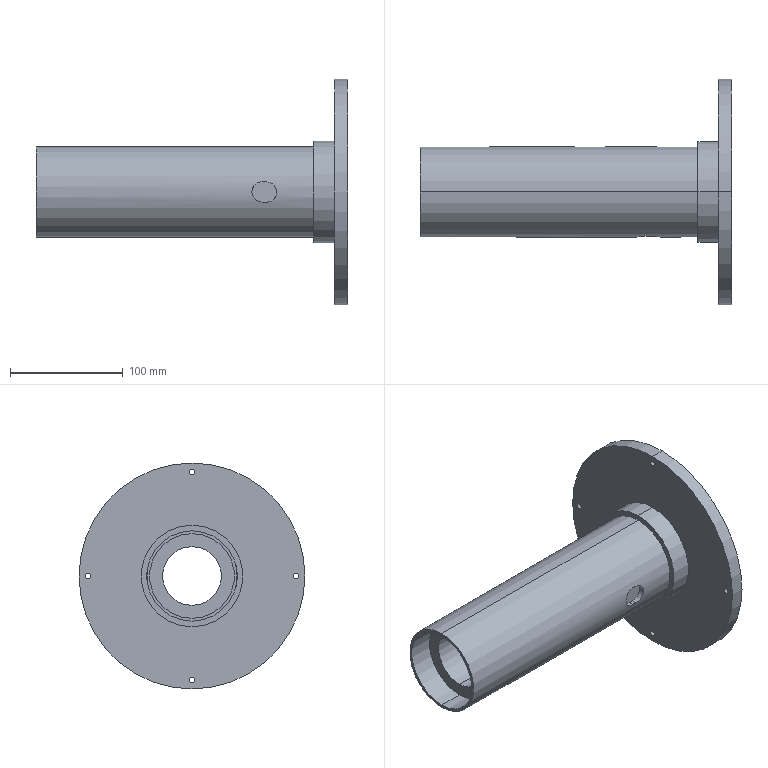Part | NX | features BREP 1 | 1 solid | 36 faces | box 276 x 200 x 200 mm | volume 1052758 mm3 | cylinder 24 | plane 12 | commonest cylinder face diameters 5 x8 9 x2 18 x2 52 x2 72 x2 75 x2
STEP:
#1=CARTESIAN_POINT('',(169.294,92.,2.5));
#2=VERTEX_POINT('',#1);
#3=CARTESIAN_POINT('',(169.294,92.,-2.5));
#4=VERTEX_POINT('',#3);
#5=CARTESIAN_POINT('',(169.294,92.,0.));
#6=DIRECTION('',(1.,0.,0.));
#7=DIRECTION('',(0.,0.,-1.));
#8=AXIS2_PLACEMENT_3D('',#5,#6,#7);
#9=CIRCLE('',#8,2.5);
#10=EDGE_CURVE('',#2,#4,#9,.T.);
#11=ORIENTED_EDGE('',*,*,#10,.F.);
#12=CARTESIAN_POINT('',(181.294,92.,2.5));
#13=VERTEX_POINT('',#12);
#14=CARTESIAN_POINT('',(181.294,92.,2.5));
#15=DIRECTION('',(1.,0.,0.));
#16=VECTOR('',#15,1000.);
#17=LINE('',#14,#16);
#18=EDGE_CURVE('',#13,#2,#17,.F.);
#19=ORIENTED_EDGE('',*,*,#18,.F.);
#20=CARTESIAN_POINT('',(181.294,92.,-2.5));
#21=VERTEX_POINT('',#20);
#22=CARTESIAN_POINT('',(181.294,92.,0.));
#23=DIRECTION('',(1.,0.,0.));
#24=DIRECTION('',(0.,0.,-1.));
#25=AXIS2_PLACEMENT_3D('',#22,#23,#24);
#26=CIRCLE('',#25,2.5);
#27=EDGE_CURVE('',#13,#21,#26,.T.);
#28=ORIENTED_EDGE('',*,*,#27,.T.);
#29=CARTESIAN_POINT('',(181.294,92.,-2.5));
#30=DIRECTION('',(1.,0.,0.));
#31=VECTOR('',#30,1000.);
#32=LINE('',#29,#31);
#33=EDGE_CURVE('',#21,#4,#32,.F.);
#34=ORIENTED_EDGE('',*,*,#33,.T.);
#35=EDGE_LOOP('',(#11,#19,#28,#34));
#36=FACE_BOUND('',#35,.T.);
#37=CARTESIAN_POINT('',(181.294,92.,0.));
#38=DIRECTION('',(1.,0.,0.));
#39=DIRECTION('',(0.,0.,1.));
#40=AXIS2_PLACEMENT_3D('',#37,#38,#39);
#41=CYLINDRICAL_SURFACE('',#40,2.5);
#42=ADVANCED_FACE('',(#36),#41,.F.);
#43=CARTESIAN_POINT('',(169.294,0.,94.5));
#44=VERTEX_POINT('',#43);
#45=CARTESIAN_POINT('',(169.294,0.,89.5));
#46=VERTEX_POINT('',#45);
#47=CARTESIAN_POINT('',(169.294,0.,92.));
#48=DIRECTION('',(1.,0.,0.));
#49=DIRECTION('',(0.,0.,-1.));
#50=AXIS2_PLACEMENT_3D('',#47,#48,#49);
#51=CIRCLE('',#50,2.5);
#52=EDGE_CURVE('',#44,#46,#51,.T.);
#53=ORIENTED_EDGE('',*,*,#52,.F.);
#54=CARTESIAN_POINT('',(181.294,0.,94.5));
#55=VERTEX_POINT('',#54);
#56=CARTESIAN_POINT('',(181.294,0.,94.5));
#57=DIRECTION('',(1.,0.,0.));
#58=VECTOR('',#57,1000.);
#59=LINE('',#56,#58);
#60=EDGE_CURVE('',#55,#44,#59,.F.);
#61=ORIENTED_EDGE('',*,*,#60,.F.);
#62=CARTESIAN_POINT('',(181.294,0.,89.5));
#63=VERTEX_POINT('',#62);
#64=CARTESIAN_POINT('',(181.294,0.,92.));
#65=DIRECTION('',(1.,0.,0.));
#66=DIRECTION('',(0.,0.,-1.));
#67=AXIS2_PLACEMENT_3D('',#64,#65,#66);
#68=CIRCLE('',#67,2.5);
#69=EDGE_CURVE('',#55,#63,#68,.T.);
#70=ORIENTED_EDGE('',*,*,#69,.T.);
#71=CARTESIAN_POINT('',(181.294,0.,89.5));
#72=DIRECTION('',(1.,0.,0.));
#73=VECTOR('',#72,1000.);
#74=LINE('',#71,#73);
#75=EDGE_CURVE('',#63,#46,#74,.F.);
#76=ORIENTED_EDGE('',*,*,#75,.T.);
#77=EDGE_LOOP('',(#53,#61,#70,#76));
#78=FACE_BOUND('',#77,.T.);
#79=CARTESIAN_POINT('',(181.294,0.,92.));
#80=DIRECTION('',(1.,0.,0.));
#81=DIRECTION('',(0.,0.,1.));
#82=AXIS2_PLACEMENT_3D('',#79,#80,#81);
#83=CYLINDRICAL_SURFACE('',#82,2.5);
#84=ADVANCED_FACE('',(#78),#83,.F.);
#85=CARTESIAN_POINT('',(169.294,0.,-89.5));
#86=VERTEX_POINT('',#85);
#87=CARTESIAN_POINT('',(169.294,0.,-94.5));
#88=VERTEX_POINT('',#87);
#89=CARTESIAN_POINT('',(169.294,0.,-92.));
#90=DIRECTION('',(1.,0.,0.));
#91=DIRECTION('',(0.,0.,-1.));
#92=AXIS2_PLACEMENT_3D('',#89,#90,#91);
#93=CIRCLE('',#92,2.5);
#94=EDGE_CURVE('',#86,#88,#93,.T.);
#95=ORIENTED_EDGE('',*,*,#94,.F.);
#96=CARTESIAN_POINT('',(181.294,0.,-89.5));
#97=VERTEX_POINT('',#96);
#98=CARTESIAN_POINT('',(181.294,0.,-89.5));
#99=DIRECTION('',(1.,0.,0.));
#100=VECTOR('',#99,1000.);
#101=LINE('',#98,#100);
#102=EDGE_CURVE('',#97,#86,#101,.F.);
#103=ORIENTED_EDGE('',*,*,#102,.F.);
#104=CARTESIAN_POINT('',(181.294,0.,-94.5));
#105=VERTEX_POINT('',#104);
#106=CARTESIAN_POINT('',(181.294,0.,-92.));
#107=DIRECTION('',(1.,0.,0.));
#108=DIRECTION('',(0.,0.,-1.));
#109=AXIS2_PLACEMENT_3D('',#106,#107,#108);
#110=CIRCLE('',#109,2.5);
#111=EDGE_CURVE('',#97,#105,#110,.T.);
#112=ORIENTED_EDGE('',*,*,#111,.T.);
#113=CARTESIAN_POINT('',(181.294,0.,-94.5));
#114=DIRECTION('',(1.,0.,0.));
#115=VECTOR('',#114,1000.);
#116=LINE('',#113,#115);
#117=EDGE_CURVE('',#105,#88,#116,.F.);
#118=ORIENTED_EDGE('',*,*,#117,.T.);
#119=EDGE_LOOP('',(#95,#103,#112,#118));
#120=FACE_BOUND('',#119,.T.);
#121=CARTESIAN_POINT('',(181.294,0.,-92.));
#122=DIRECTION('',(1.,0.,0.));
#123=DIRECTION('',(0.,0.,1.));
#124=AXIS2_PLACEMENT_3D('',#121,#122,#123);
#125=CYLINDRICAL_SURFACE('',#124,2.5);
#126=ADVANCED_FACE('',(#120),#125,.F.);
#127=CARTESIAN_POINT('',(169.294,-92.,2.5));
#128=VERTEX_POINT('',#127);
#129=CARTESIAN_POINT('',(169.294,-92.,-2.5));
#130=VERTEX_POINT('',#129);
#131=CARTESIAN_POINT('',(169.294,-92.,0.));
#132=DIRECTION('',(1.,0.,0.));
#133=DIRECTION('',(0.,0.,-1.));
#134=AXIS2_PLACEMENT_3D('',#131,#132,#133);
#135=CIRCLE('',#134,2.5);
#136=EDGE_CURVE('',#128,#130,#135,.T.);
#137=ORIENTED_EDGE('',*,*,#136,.F.);
#138=CARTESIAN_POINT('',(181.294,-92.,2.5));
#139=VERTEX_POINT('',#138);
#140=CARTESIAN_POINT('',(181.294,-92.,2.5));
#141=DIRECTION('',(1.,0.,0.));
#142=VECTOR('',#141,1000.);
#143=LINE('',#140,#142);
#144=EDGE_CURVE('',#139,#128,#143,.F.);
#145=ORIENTED_EDGE('',*,*,#144,.F.);
#146=CARTESIAN_POINT('',(181.294,-92.,-2.5));
#147=VERTEX_POINT('',#146);
#148=CARTESIAN_POINT('',(181.294,-92.,0.));
#149=DIRECTION('',(1.,0.,0.));
#150=DIRECTION('',(0.,0.,-1.));
#151=AXIS2_PLACEMENT_3D('',#148,#149,#150);
#152=CIRCLE('',#151,2.5);
#153=EDGE_CURVE('',#139,#147,#152,.T.);
#154=ORIENTED_EDGE('',*,*,#153,.T.);
#155=CARTESIAN_POINT('',(181.294,-92.,-2.5));
#156=DIRECTION('',(1.,0.,0.));
#157=VECTOR('',#156,1000.);
#158=LINE('',#155,#157);
#159=EDGE_CURVE('',#147,#130,#158,.F.);
#160=ORIENTED_EDGE('',*,*,#159,.T.);
#161=EDGE_LOOP('',(#137,#145,#154,#160));
#162=FACE_BOUND('',#161,.T.);
#163=CARTESIAN_POINT('',(181.294,-92.,0.));
#164=DIRECTION('',(1.,0.,0.));
#165=DIRECTION('',(0.,0.,1.));
#166=AXIS2_PLACEMENT_3D('',#163,#164,#165);
#167=CYLINDRICAL_SURFACE('',#166,2.5);
#168=ADVANCED_FACE('',(#162),#167,.F.);
#169=CARTESIAN_POINT('',(169.294,0.,45.));
#170=VERTEX_POINT('',#169);
#171=CARTESIAN_POINT('',(169.294,0.,-45.));
#172=VERTEX_POINT('',#171);
#173=CARTESIAN_POINT('',(169.294,0.,0.));
#174=DIRECTION('',(-1.,0.,0.));
#175=DIRECTION('',(0.,0.,1.));
#176=AXIS2_PLACEMENT_3D('',#173,#174,#175);
#177=CIRCLE('',#176,45.);
#178=EDGE_CURVE('',#170,#172,#177,.T.);
#179=ORIENTED_EDGE('',*,*,#178,.T.);
#180=CARTESIAN_POINT('',(151.294,0.,-45.));
#181=VERTEX_POINT('',#180);
#182=CARTESIAN_POINT('',(-170.105,0.,-45.));
#183=DIRECTION('',(-1.,0.,0.));
#184=VECTOR('',#183,1000.);
#185=LINE('',#182,#184);
#186=EDGE_CURVE('',#172,#181,#185,.T.);
#187=ORIENTED_EDGE('',*,*,#186,.T.);
#188=CARTESIAN_POINT('',(151.294,0.,45.));
#189=VERTEX_POINT('',#188);
#190=CARTESIAN_POINT('',(151.294,0.,0.));
#191=DIRECTION('',(-1.,0.,0.));
#192=DIRECTION('',(0.,0.,1.));
#193=AXIS2_PLACEMENT_3D('',#190,#191,#192);
#194=CIRCLE('',#193,45.);
#195=EDGE_CURVE('',#189,#181,#194,.T.);
#196=ORIENTED_EDGE('',*,*,#195,.F.);
#197=CARTESIAN_POINT('',(-170.105,0.,45.));
#198=DIRECTION('',(-1.,0.,0.));
#199=VECTOR('',#198,1000.);
#200=LINE('',#197,#199);
#201=EDGE_CURVE('',#170,#189,#200,.T.);
#202=ORIENTED_EDGE('',*,*,#201,.F.);
#203=EDGE_LOOP('',(#179,#187,#196,#202));
#204=FACE_BOUND('',#203,.T.);
#205=CARTESIAN_POINT('',(-170.105,0.,0.));
#206=DIRECTION('',(-1.,0.,0.));
#207=DIRECTION('',(0.,0.,-1.));
#208=AXIS2_PLACEMENT_3D('',#205,#206,#207);
#209=CYLINDRICAL_SURFACE('',#208,45.);
#210=ADVANCED_FACE('',(#204),#209,.T.);
#211=CARTESIAN_POINT('',(181.294,0.,100.));
#212=VERTEX_POINT('',#211);
#213=CARTESIAN_POINT('',(181.294,0.,-100.));
#214=VERTEX_POINT('',#213);
#215=CARTESIAN_POINT('',(181.294,0.,0.));
#216=DIRECTION('',(-1.,0.,0.));
#217=DIRECTION('',(0.,0.,1.));
#218=AXIS2_PLACEMENT_3D('',#215,#216,#217);
#219=CIRCLE('',#218,100.);
#220=EDGE_CURVE('',#212,#214,#219,.T.);
#221=ORIENTED_EDGE('',*,*,#220,.T.);
#222=CARTESIAN_POINT('',(169.294,0.,-100.));
#223=VERTEX_POINT('',#222);
#224=CARTESIAN_POINT('',(-170.105,0.,-100.));
#225=DIRECTION('',(-1.,0.,0.));
#226=VECTOR('',#225,1000.);
#227=LINE('',#224,#226);
#228=EDGE_CURVE('',#214,#223,#227,.T.);
#229=ORIENTED_EDGE('',*,*,#228,.T.);
#230=CARTESIAN_POINT('',(169.294,0.,100.));
#231=VERTEX_POINT('',#230);
#232=CARTESIAN_POINT('',(169.294,0.,0.));
#233=DIRECTION('',(-1.,0.,0.));
#234=DIRECTION('',(0.,0.,1.));
#235=AXIS2_PLACEMENT_3D('',#232,#233,#234);
#236=CIRCLE('',#235,100.);
#237=EDGE_CURVE('',#231,#223,#236,.T.);
#238=ORIENTED_EDGE('',*,*,#237,.F.);
#239=CARTESIAN_POINT('',(-170.105,0.,100.));
#240=DIRECTION('',(-1.,0.,0.));
#241=VECTOR('',#240,1000.);
#242=LINE('',#239,#241);
#243=EDGE_CURVE('',#212,#231,#242,.T.);
#244=ORIENTED_EDGE('',*,*,#243,.F.);
#245=EDGE_LOOP('',(#221,#229,#238,#244));
#246=FACE_BOUND('',#245,.T.);
#247=CARTESIAN_POINT('',(-170.105,0.,0.));
#248=DIRECTION('',(-1.,0.,0.));
#249=DIRECTION('',(0.,0.,-1.));
#250=AXIS2_PLACEMENT_3D('',#247,#248,#249);
#251=CYLINDRICAL_SURFACE('',#250,100.);
#252=ADVANCED_FACE('',(#246),#251,.T.);
#253=CARTESIAN_POINT('',(181.294,0.,-36.));
#254=VERTEX_POINT('',#253);
#255=CARTESIAN_POINT('',(181.294,0.,36.));
#256=VERTEX_POINT('',#255);
#257=CARTESIAN_POINT('',(181.294,0.,0.));
#258=DIRECTION('',(-1.,0.,0.));
#259=DIRECTION('',(0.,0.,1.));
#260=AXIS2_PLACEMENT_3D('',#257,#258,#259);
#261=CIRCLE('',#260,36.);
#262=EDGE_CURVE('',#254,#256,#261,.T.);
#263=ORIENTED_EDGE('',*,*,#262,.F.);
#264=CARTESIAN_POINT('',(163.294,0.,-36.));
#265=VERTEX_POINT('',#264);
#266=CARTESIAN_POINT('',(-170.105,0.,-36.));
#267=DIRECTION('',(-1.,0.,0.));
#268=VECTOR('',#267,1000.);
#269=LINE('',#266,#268);
#270=EDGE_CURVE('',#254,#265,#269,.T.);
#271=ORIENTED_EDGE('',*,*,#270,.T.);
#272=CARTESIAN_POINT('',(163.294,0.,36.));
#273=VERTEX_POINT('',#272);
#274=CARTESIAN_POINT('',(163.294,0.,0.));
#275=DIRECTION('',(-1.,0.,0.));
#276=DIRECTION('',(0.,0.,1.));
#277=AXIS2_PLACEMENT_3D('',#274,#275,#276);
#278=CIRCLE('',#277,36.);
#279=EDGE_CURVE('',#265,#273,#278,.T.);
#280=ORIENTED_EDGE('',*,*,#279,.T.);
#281=CARTESIAN_POINT('',(-170.105,0.,36.));
#282=DIRECTION('',(-1.,0.,0.));
#283=VECTOR('',#282,1000.);
#284=LINE('',#281,#283);
#285=EDGE_CURVE('',#256,#273,#284,.T.);
#286=ORIENTED_EDGE('',*,*,#285,.F.);
#287=EDGE_LOOP('',(#263,#271,#280,#286));
#288=FACE_BOUND('',#287,.T.);
#289=CARTESIAN_POINT('',(-170.105,0.,0.));
#290=DIRECTION('',(-1.,0.,0.));
#291=DIRECTION('',(0.,0.,-1.));
#292=AXIS2_PLACEMENT_3D('',#289,#290,#291);
#293=CYLINDRICAL_SURFACE('',#292,36.);
#294=ADVANCED_FACE('',(#288),#293,.F.);
#295=CARTESIAN_POINT('',(163.294,0.,-26.));
#296=VERTEX_POINT('',#295);
#297=CARTESIAN_POINT('',(163.294,0.,26.));
#298=VERTEX_POINT('',#297);
#299=CARTESIAN_POINT('',(163.294,0.,0.));
#300=DIRECTION('',(-1.,0.,0.));
#301=DIRECTION('',(0.,0.,1.));
#302=AXIS2_PLACEMENT_3D('',#299,#300,#301);
#303=CIRCLE('',#302,26.);
#304=EDGE_CURVE('',#296,#298,#303,.T.);
#305=ORIENTED_EDGE('',*,*,#304,.F.);
#306=CARTESIAN_POINT('',(-72.706,0.,-26.));
#307=VERTEX_POINT('',#306);
#308=CARTESIAN_POINT('',(-170.105,0.,-26.));
#309=DIRECTION('',(-1.,0.,0.));
#310=VECTOR('',#309,1000.);
#311=LINE('',#308,#310);
#312=EDGE_CURVE('',#296,#307,#311,.T.);
#313=ORIENTED_EDGE('',*,*,#312,.T.);
#314=CARTESIAN_POINT('',(-72.706,0.,26.));
#315=VERTEX_POINT('',#314);
#316=CARTESIAN_POINT('',(-72.706,0.,0.));
#317=DIRECTION('',(-1.,0.,0.));
#318=DIRECTION('',(0.,0.,1.));
#319=AXIS2_PLACEMENT_3D('',#316,#317,#318);
#320=CIRCLE('',#319,26.);
#321=EDGE_CURVE('',#307,#315,#320,.T.);
#322=ORIENTED_EDGE('',*,*,#321,.T.);
#323=CARTESIAN_POINT('',(-170.105,0.,26.));
#324=DIRECTION('',(-1.,0.,0.));
#325=VECTOR('',#324,1000.);
#326=LINE('',#323,#325);
#327=EDGE_CURVE('',#298,#315,#326,.T.);
#328=ORIENTED_EDGE('',*,*,#327,.F.);
#329=EDGE_LOOP('',(#305,#313,#322,#328));
#330=FACE_BOUND('',#329,.T.);
#331=CARTESIAN_POINT('',(-170.105,0.,0.));
#332=DIRECTION('',(-1.,0.,0.));
#333=DIRECTION('',(0.,0.,-1.));
#334=AXIS2_PLACEMENT_3D('',#331,#332,#333);
#335=CYLINDRICAL_SURFACE('',#334,26.);
#336=ADVANCED_FACE('',(#330),#335,.F.);
#337=CARTESIAN_POINT('',(-72.706,0.,-37.5));
#338=VERTEX_POINT('',#337);
#339=CARTESIAN_POINT('',(-72.706,0.,37.5));
#340=VERTEX_POINT('',#339);
#341=CARTESIAN_POINT('',(-72.706,0.,0.));
#342=DIRECTION('',(-1.,0.,0.));
#343=DIRECTION('',(0.,0.,1.));
#344=AXIS2_PLACEMENT_3D('',#341,#342,#343);
#345=CIRCLE('',#344,37.5);
#346=EDGE_CURVE('',#338,#340,#345,.T.);
#347=ORIENTED_EDGE('',*,*,#346,.F.);
#348=CARTESIAN_POINT('',(-94.706,0.,-37.5));
#349=VERTEX_POINT('',#348);
#350=CARTESIAN_POINT('',(-170.105,0.,-37.5));
#351=DIRECTION('',(-1.,0.,0.));
#352=VECTOR('',#351,1000.);
#353=LINE('',#350,#352);
#354=EDGE_CURVE('',#338,#349,#353,.T.);
#355=ORIENTED_EDGE('',*,*,#354,.T.);
#356=CARTESIAN_POINT('',(-94.706,0.,37.5));
#357=VERTEX_POINT('',#356);
#358=CARTESIAN_POINT('',(-94.706,0.,0.));
#359=DIRECTION('',(-1.,0.,0.));
#360=DIRECTION('',(0.,0.,1.));
#361=AXIS2_PLACEMENT_3D('',#358,#359,#360);
#362=CIRCLE('',#361,37.5);
#363=EDGE_CURVE('',#349,#357,#362,.T.);
#364=ORIENTED_EDGE('',*,*,#363,.T.);
#365=CARTESIAN_POINT('',(-170.105,0.,37.5));
#366=DIRECTION('',(-1.,0.,0.));
#367=VECTOR('',#366,1000.);
#368=LINE('',#365,#367);
#369=EDGE_CURVE('',#340,#357,#368,.T.);
#370=ORIENTED_EDGE('',*,*,#369,.F.);
#371=EDGE_LOOP('',(#347,#355,#364,#370));
#372=FACE_BOUND('',#371,.T.);
#373=CARTESIAN_POINT('',(-170.105,0.,0.));
#374=DIRECTION('',(-1.,0.,0.));
#375=DIRECTION('',(0.,0.,-1.));
#376=AXIS2_PLACEMENT_3D('',#373,#374,#375);
#377=CYLINDRICAL_SURFACE('',#376,37.5);
#378=ADVANCED_FACE('',(#372),#377,.F.);
#379=CARTESIAN_POINT('',(151.294,0.,40.));
#380=VERTEX_POINT('',#379);
#381=CARTESIAN_POINT('',(151.294,0.,-40.));
#382=VERTEX_POINT('',#381);
#383=CARTESIAN_POINT('',(151.294,0.,0.));
#384=DIRECTION('',(-1.,0.,0.));
#385=DIRECTION('',(0.,0.,1.));
#386=AXIS2_PLACEMENT_3D('',#383,#384,#385);
#387=CIRCLE('',#386,40.);
#388=EDGE_CURVE('',#380,#382,#387,.T.);
#389=ORIENTED_EDGE('',*,*,#388,.T.);
#390=CARTESIAN_POINT('',(-94.706,0.,-40.));
#391=VERTEX_POINT('',#390);
#392=CARTESIAN_POINT('',(-170.105,0.,-40.));
#393=DIRECTION('',(-1.,0.,0.));
#394=VECTOR('',#393,1000.);
#395=LINE('',#392,#394);
#396=EDGE_CURVE('',#382,#391,#395,.T.);
#397=ORIENTED_EDGE('',*,*,#396,.T.);
#398=CARTESIAN_POINT('',(-94.706,0.,40.));
#399=VERTEX_POINT('',#398);
#400=CARTESIAN_POINT('',(-94.706,0.,0.));
#401=DIRECTION('',(-1.,0.,0.));
#402=DIRECTION('',(0.,0.,1.));
#403=AXIS2_PLACEMENT_3D('',#400,#401,#402);
#404=CIRCLE('',#403,40.);
#405=EDGE_CURVE('',#399,#391,#404,.T.);
#406=ORIENTED_EDGE('',*,*,#405,.F.);
#407=CARTESIAN_POINT('',(-170.105,0.,40.));
#408=DIRECTION('',(-1.,0.,0.));
#409=VECTOR('',#408,1000.);
#410=LINE('',#407,#409);
#411=EDGE_CURVE('',#380,#399,#410,.T.);
#412=ORIENTED_EDGE('',*,*,#411,.F.);
#413=EDGE_LOOP('',(#389,#397,#406,#412));
#414=FACE_BOUND('',#413,.T.);
#415=CARTESIAN_POINT('',(45.294,39.746,-4.5));
#416=VERTEX_POINT('',#415);
#417=CARTESIAN_POINT('',(66.294,39.746,-4.5));
#418=VERTEX_POINT('',#417);
#419=CARTESIAN_POINT('',(-170.105,39.746,-4.5));
#420=DIRECTION('',(1.,0.,0.));
#421=VECTOR('',#420,1000.);
#422=LINE('',#419,#421);
#423=EDGE_CURVE('',#416,#418,#422,.T.);
#424=ORIENTED_EDGE('',*,*,#423,.T.);
#425=CARTESIAN_POINT('',(66.294,39.746,4.5));
#426=VERTEX_POINT('',#425);
#427=CARTESIAN_POINT('',(66.294,39.746,-4.5));
#428=CARTESIAN_POINT('',(67.484,39.746,-4.5));
#429=CARTESIAN_POINT('',(69.813,39.873,-3.525));
#430=CARTESIAN_POINT('',(71.283,40.063,-0.00463));
#431=CARTESIAN_POINT('',(69.816,39.874,3.524));
#432=CARTESIAN_POINT('',(67.484,39.746,4.5));
#433=CARTESIAN_POINT('',(66.294,39.746,4.5));
#434=B_SPLINE_CURVE_WITH_KNOTS('',3,(#427,#428,#429,#430,#431,#432,#433),.UNSPECIFIED.,.F.,.F.,(4,1,1,1,4),(0.,0.003519,0.007039,0.01056,0.01408),.UNSPECIFIED.);
#435=EDGE_CURVE('',#418,#426,#434,.T.);
#436=ORIENTED_EDGE('',*,*,#435,.T.);
#437=CARTESIAN_POINT('',(45.294,39.746,4.5));
#438=VERTEX_POINT('',#437);
#439=CARTESIAN_POINT('',(-170.105,39.746,4.5));
#440=DIRECTION('',(-1.,0.,0.));
#441=VECTOR('',#440,1000.);
#442=LINE('',#439,#441);
#443=EDGE_CURVE('',#426,#438,#442,.T.);
#444=ORIENTED_EDGE('',*,*,#443,.T.);
#445=CARTESIAN_POINT('',(45.294,39.746,4.5));
#446=CARTESIAN_POINT('',(44.104,39.746,4.5));
#447=CARTESIAN_POINT('',(41.774,39.873,3.525));
#448=CARTESIAN_POINT('',(40.304,40.063,0.00463));
#449=CARTESIAN_POINT('',(41.771,39.874,-3.524));
#450=CARTESIAN_POINT('',(44.104,39.746,-4.5));
#451=CARTESIAN_POINT('',(45.294,39.746,-4.5));
#452=B_SPLINE_CURVE_WITH_KNOTS('',3,(#445,#446,#447,#448,#449,#450,#451),.UNSPECIFIED.,.F.,.F.,(4,1,1,1,4),(0.,0.003519,0.007039,0.01056,0.01408),.UNSPECIFIED.);
#453=EDGE_CURVE('',#438,#416,#452,.T.);
#454=ORIENTED_EDGE('',*,*,#453,.T.);
#455=EDGE_LOOP('',(#424,#436,#444,#454));
#456=FACE_BOUND('',#455,.T.);
#457=CARTESIAN_POINT('',(-170.105,0.,0.));
#458=DIRECTION('',(-1.,0.,0.));
#459=DIRECTION('',(0.,0.,-1.));
#460=AXIS2_PLACEMENT_3D('',#457,#458,#459);
#461=CYLINDRICAL_SURFACE('',#460,40.);
#462=ADVANCED_FACE('',(#414,#456),#461,.T.);
#463=ORIENTED_EDGE('',*,*,#220,.F.);
#464=CARTESIAN_POINT('',(181.294,0.,0.));
#465=DIRECTION('',(-1.,0.,0.));
#466=DIRECTION('',(0.,0.,1.));
#467=AXIS2_PLACEMENT_3D('',#464,#465,#466);
#468=CIRCLE('',#467,100.);
#469=EDGE_CURVE('',#214,#212,#468,.T.);
#470=ORIENTED_EDGE('',*,*,#469,.F.);
#471=EDGE_LOOP('',(#463,#470));
#472=FACE_BOUND('',#471,.T.);
#473=CARTESIAN_POINT('',(181.294,0.,0.));
#474=DIRECTION('',(-1.,0.,0.));
#475=DIRECTION('',(0.,0.,1.));
#476=AXIS2_PLACEMENT_3D('',#473,#474,#475);
#477=CIRCLE('',#476,36.);
#478=EDGE_CURVE('',#256,#254,#477,.T.);
#479=ORIENTED_EDGE('',*,*,#478,.T.);
#480=ORIENTED_EDGE('',*,*,#262,.T.);
#481=EDGE_LOOP('',(#479,#480));
#482=FACE_BOUND('',#481,.T.);
#483=CARTESIAN_POINT('',(181.294,-92.,0.));
#484=DIRECTION('',(1.,0.,0.));
#485=DIRECTION('',(0.,0.,-1.));
#486=AXIS2_PLACEMENT_3D('',#483,#484,#485);
#487=CIRCLE('',#486,2.5);
#488=EDGE_CURVE('',#147,#139,#487,.T.);
#489=ORIENTED_EDGE('',*,*,#488,.F.);
#490=ORIENTED_EDGE('',*,*,#153,.F.);
#491=EDGE_LOOP('',(#489,#490));
#492=FACE_BOUND('',#491,.T.);
#493=CARTESIAN_POINT('',(181.294,0.,-92.));
#494=DIRECTION('',(1.,0.,0.));
#495=DIRECTION('',(0.,0.,-1.));
#496=AXIS2_PLACEMENT_3D('',#493,#494,#495);
#497=CIRCLE('',#496,2.5);
#498=EDGE_CURVE('',#105,#97,#497,.T.);
#499=ORIENTED_EDGE('',*,*,#498,.F.);
#500=ORIENTED_EDGE('',*,*,#111,.F.);
#501=EDGE_LOOP('',(#499,#500));
#502=FACE_BOUND('',#501,.T.);
#503=CARTESIAN_POINT('',(181.294,0.,92.));
#504=DIRECTION('',(1.,0.,0.));
#505=DIRECTION('',(0.,0.,-1.));
#506=AXIS2_PLACEMENT_3D('',#503,#504,#505);
#507=CIRCLE('',#506,2.5);
#508=EDGE_CURVE('',#63,#55,#507,.T.);
#509=ORIENTED_EDGE('',*,*,#508,.F.);
#510=ORIENTED_EDGE('',*,*,#69,.F.);
#511=EDGE_LOOP('',(#509,#510));
#512=FACE_BOUND('',#511,.T.);
#513=CARTESIAN_POINT('',(181.294,92.,0.));
#514=DIRECTION('',(1.,0.,0.));
#515=DIRECTION('',(0.,0.,-1.));
#516=AXIS2_PLACEMENT_3D('',#513,#514,#515);
#517=CIRCLE('',#516,2.5);
#518=EDGE_CURVE('',#21,#13,#517,.T.);
#519=ORIENTED_EDGE('',*,*,#518,.F.);
#520=ORIENTED_EDGE('',*,*,#27,.F.);
#521=EDGE_LOOP('',(#519,#520));
#522=FACE_BOUND('',#521,.T.);
#523=CARTESIAN_POINT('',(181.294,100.,0.));
#524=DIRECTION('',(-1.,0.,0.));
#525=DIRECTION('',(0.,-1.,0.));
#526=AXIS2_PLACEMENT_3D('',#523,#524,#525);
#527=PLANE('',#526);
#528=ADVANCED_FACE('',(#472,#482,#492,#502,#512,#522),#527,.F.);
#529=ORIENTED_EDGE('',*,*,#396,.F.);
#530=CARTESIAN_POINT('',(151.294,0.,0.));
#531=DIRECTION('',(-1.,0.,0.));
#532=DIRECTION('',(0.,0.,1.));
#533=AXIS2_PLACEMENT_3D('',#530,#531,#532);
#534=CIRCLE('',#533,40.);
#535=EDGE_CURVE('',#382,#380,#534,.T.);
#536=ORIENTED_EDGE('',*,*,#535,.T.);
#537=ORIENTED_EDGE('',*,*,#411,.T.);
#538=CARTESIAN_POINT('',(-94.706,0.,0.));
#539=DIRECTION('',(-1.,0.,0.));
#540=DIRECTION('',(0.,0.,1.));
#541=AXIS2_PLACEMENT_3D('',#538,#539,#540);
#542=CIRCLE('',#541,40.);
#543=EDGE_CURVE('',#391,#399,#542,.T.);
#544=ORIENTED_EDGE('',*,*,#543,.F.);
#545=EDGE_LOOP('',(#529,#536,#537,#544));
#546=FACE_BOUND('',#545,.T.);
#547=CARTESIAN_POINT('',(109.294,-38.974,-9.));
#548=VERTEX_POINT('',#547);
#549=CARTESIAN_POINT('',(109.294,-38.974,9.));
#550=VERTEX_POINT('',#549);
#551=CARTESIAN_POINT('',(109.294,-38.974,-9.));
#552=CARTESIAN_POINT('',(111.68,-38.974,-9.));
#553=CARTESIAN_POINT('',(116.329,-39.494,-7.049));
#554=CARTESIAN_POINT('',(119.275,-40.253,-0.01185));
#555=CARTESIAN_POINT('',(116.334,-39.495,7.051));
#556=CARTESIAN_POINT('',(111.68,-38.974,9.));
#557=CARTESIAN_POINT('',(109.294,-38.974,9.));
#558=B_SPLINE_CURVE_WITH_KNOTS('',3,(#551,#552,#553,#554,#555,#556,#557),.UNSPECIFIED.,.F.,.F.,(4,1,1,1,4),(0.,0.007055,0.01411,0.02117,0.02822),.UNSPECIFIED.);
#559=EDGE_CURVE('',#548,#550,#558,.T.);
#560=ORIENTED_EDGE('',*,*,#559,.F.);
#561=CARTESIAN_POINT('',(105.294,-38.974,-9.));
#562=VERTEX_POINT('',#561);
#563=CARTESIAN_POINT('',(-170.105,-38.974,-9.));
#564=DIRECTION('',(1.,0.,0.));
#565=VECTOR('',#564,1000.);
#566=LINE('',#563,#565);
#567=EDGE_CURVE('',#562,#548,#566,.T.);
#568=ORIENTED_EDGE('',*,*,#567,.F.);
#569=CARTESIAN_POINT('',(105.294,-38.974,9.));
#570=VERTEX_POINT('',#569);
#571=CARTESIAN_POINT('',(105.294,-38.974,9.));
#572=CARTESIAN_POINT('',(102.907,-38.974,9.));
#573=CARTESIAN_POINT('',(98.258,-39.494,7.049));
#574=CARTESIAN_POINT('',(95.312,-40.253,0.01185));
#575=CARTESIAN_POINT('',(98.253,-39.495,-7.051));
#576=CARTESIAN_POINT('',(102.907,-38.974,-9.));
#577=CARTESIAN_POINT('',(105.294,-38.974,-9.));
#578=B_SPLINE_CURVE_WITH_KNOTS('',3,(#571,#572,#573,#574,#575,#576,#577),.UNSPECIFIED.,.F.,.F.,(4,1,1,1,4),(0.,0.007055,0.01411,0.02117,0.02822),.UNSPECIFIED.);
#579=EDGE_CURVE('',#570,#562,#578,.T.);
#580=ORIENTED_EDGE('',*,*,#579,.F.);
#581=CARTESIAN_POINT('',(-170.105,-38.974,9.));
#582=DIRECTION('',(-1.,0.,0.));
#583=VECTOR('',#582,1000.);
#584=LINE('',#581,#583);
#585=EDGE_CURVE('',#550,#570,#584,.T.);
#586=ORIENTED_EDGE('',*,*,#585,.F.);
#587=EDGE_LOOP('',(#560,#568,#580,#586));
#588=FACE_BOUND('',#587,.T.);
#589=CARTESIAN_POINT('',(-170.105,0.,0.));
#590=DIRECTION('',(-1.,0.,0.));
#591=DIRECTION('',(0.,0.,-1.));
#592=AXIS2_PLACEMENT_3D('',#589,#590,#591);
#593=CYLINDRICAL_SURFACE('',#592,40.);
#594=ADVANCED_FACE('',(#546,#588),#593,.T.);
#595=ORIENTED_EDGE('',*,*,#405,.T.);
#596=ORIENTED_EDGE('',*,*,#543,.T.);
#597=EDGE_LOOP('',(#595,#596));
#598=FACE_BOUND('',#597,.T.);
#599=CARTESIAN_POINT('',(-94.706,0.,0.));
#600=DIRECTION('',(-1.,0.,0.));
#601=DIRECTION('',(0.,0.,1.));
#602=AXIS2_PLACEMENT_3D('',#599,#600,#601);
#603=CIRCLE('',#602,37.5);
#604=EDGE_CURVE('',#357,#349,#603,.T.);
#605=ORIENTED_EDGE('',*,*,#604,.F.);
#606=ORIENTED_EDGE('',*,*,#363,.F.);
#607=EDGE_LOOP('',(#605,#606));
#608=FACE_BOUND('',#607,.T.);
#609=CARTESIAN_POINT('',(-94.706,37.5,0.));
#610=DIRECTION('',(1.,0.,0.));
#611=DIRECTION('',(0.,0.,1.));
#612=AXIS2_PLACEMENT_3D('',#609,#610,#611);
#613=PLANE('',#612);
#614=ADVANCED_FACE('',(#598,#608),#613,.F.);
#615=ORIENTED_EDGE('',*,*,#354,.F.);
#616=CARTESIAN_POINT('',(-72.706,0.,0.));
#617=DIRECTION('',(-1.,0.,0.));
#618=DIRECTION('',(0.,0.,1.));
#619=AXIS2_PLACEMENT_3D('',#616,#617,#618);
#620=CIRCLE('',#619,37.5);
#621=EDGE_CURVE('',#340,#338,#620,.T.);
#622=ORIENTED_EDGE('',*,*,#621,.F.);
#623=ORIENTED_EDGE('',*,*,#369,.T.);
#624=ORIENTED_EDGE('',*,*,#604,.T.);
#625=EDGE_LOOP('',(#615,#622,#623,#624));
#626=FACE_BOUND('',#625,.T.);
#627=CARTESIAN_POINT('',(-170.105,0.,0.));
#628=DIRECTION('',(-1.,0.,0.));
#629=DIRECTION('',(0.,0.,-1.));
#630=AXIS2_PLACEMENT_3D('',#627,#628,#629);
#631=CYLINDRICAL_SURFACE('',#630,37.5);
#632=ADVANCED_FACE('',(#626),#631,.F.);
#633=ORIENTED_EDGE('',*,*,#621,.T.);
#634=ORIENTED_EDGE('',*,*,#346,.T.);
#635=EDGE_LOOP('',(#633,#634));
#636=FACE_BOUND('',#635,.T.);
#637=CARTESIAN_POINT('',(-72.706,0.,0.));
#638=DIRECTION('',(-1.,0.,0.));
#639=DIRECTION('',(0.,0.,1.));
#640=AXIS2_PLACEMENT_3D('',#637,#638,#639);
#641=CIRCLE('',#640,26.);
#642=EDGE_CURVE('',#315,#307,#641,.T.);
#643=ORIENTED_EDGE('',*,*,#642,.F.);
#644=ORIENTED_EDGE('',*,*,#321,.F.);
#645=EDGE_LOOP('',(#643,#644));
#646=FACE_BOUND('',#645,.T.);
#647=CARTESIAN_POINT('',(-72.706,37.5,0.));
#648=DIRECTION('',(1.,0.,0.));
#649=DIRECTION('',(0.,0.,1.));
#650=AXIS2_PLACEMENT_3D('',#647,#648,#649);
#651=PLANE('',#650);
#652=ADVANCED_FACE('',(#636,#646),#651,.F.);
#653=ORIENTED_EDGE('',*,*,#312,.F.);
#654=CARTESIAN_POINT('',(163.294,0.,0.));
#655=DIRECTION('',(-1.,0.,0.));
#656=DIRECTION('',(0.,0.,1.));
#657=AXIS2_PLACEMENT_3D('',#654,#655,#656);
#658=CIRCLE('',#657,26.);
#659=EDGE_CURVE('',#298,#296,#658,.T.);
#660=ORIENTED_EDGE('',*,*,#659,.F.);
#661=ORIENTED_EDGE('',*,*,#327,.T.);
#662=ORIENTED_EDGE('',*,*,#642,.T.);
#663=EDGE_LOOP('',(#653,#660,#661,#662));
#664=FACE_BOUND('',#663,.T.);
#665=CARTESIAN_POINT('',(-170.105,0.,0.));
#666=DIRECTION('',(-1.,0.,0.));
#667=DIRECTION('',(0.,0.,-1.));
#668=AXIS2_PLACEMENT_3D('',#665,#666,#667);
#669=CYLINDRICAL_SURFACE('',#668,26.);
#670=ADVANCED_FACE('',(#664),#669,.F.);
#671=CARTESIAN_POINT('',(163.294,0.,0.));
#672=DIRECTION('',(-1.,0.,0.));
#673=DIRECTION('',(0.,0.,1.));
#674=AXIS2_PLACEMENT_3D('',#671,#672,#673);
#675=CIRCLE('',#674,36.);
#676=EDGE_CURVE('',#273,#265,#675,.T.);
#677=ORIENTED_EDGE('',*,*,#676,.F.);
#678=ORIENTED_EDGE('',*,*,#279,.F.);
#679=EDGE_LOOP('',(#677,#678));
#680=FACE_BOUND('',#679,.T.);
#681=ORIENTED_EDGE('',*,*,#659,.T.);
#682=ORIENTED_EDGE('',*,*,#304,.T.);
#683=EDGE_LOOP('',(#681,#682));
#684=FACE_BOUND('',#683,.T.);
#685=CARTESIAN_POINT('',(163.294,36.,0.));
#686=DIRECTION('',(-1.,0.,0.));
#687=DIRECTION('',(0.,-1.,0.));
#688=AXIS2_PLACEMENT_3D('',#685,#686,#687);
#689=PLANE('',#688);
#690=ADVANCED_FACE('',(#680,#684),#689,.F.);
#691=ORIENTED_EDGE('',*,*,#270,.F.);
#692=ORIENTED_EDGE('',*,*,#478,.F.);
#693=ORIENTED_EDGE('',*,*,#285,.T.);
#694=ORIENTED_EDGE('',*,*,#676,.T.);
#695=EDGE_LOOP('',(#691,#692,#693,#694));
#696=FACE_BOUND('',#695,.T.);
#697=CARTESIAN_POINT('',(-170.105,0.,0.));
#698=DIRECTION('',(-1.,0.,0.));
#699=DIRECTION('',(0.,0.,-1.));
#700=AXIS2_PLACEMENT_3D('',#697,#698,#699);
#701=CYLINDRICAL_SURFACE('',#700,36.);
#702=ADVANCED_FACE('',(#696),#701,.F.);
#703=ORIENTED_EDGE('',*,*,#228,.F.);
#704=ORIENTED_EDGE('',*,*,#469,.T.);
#705=ORIENTED_EDGE('',*,*,#243,.T.);
#706=CARTESIAN_POINT('',(169.294,0.,0.));
#707=DIRECTION('',(-1.,0.,0.));
#708=DIRECTION('',(0.,0.,1.));
#709=AXIS2_PLACEMENT_3D('',#706,#707,#708);
#710=CIRCLE('',#709,100.);
#711=EDGE_CURVE('',#223,#231,#710,.T.);
#712=ORIENTED_EDGE('',*,*,#711,.F.);
#713=EDGE_LOOP('',(#703,#704,#705,#712));
#714=FACE_BOUND('',#713,.T.);
#715=CARTESIAN_POINT('',(-170.105,0.,0.));
#716=DIRECTION('',(-1.,0.,0.));
#717=DIRECTION('',(0.,0.,-1.));
#718=AXIS2_PLACEMENT_3D('',#715,#716,#717);
#719=CYLINDRICAL_SURFACE('',#718,100.);
#720=ADVANCED_FACE('',(#714),#719,.T.);
#721=ORIENTED_EDGE('',*,*,#237,.T.);
#722=ORIENTED_EDGE('',*,*,#711,.T.);
#723=EDGE_LOOP('',(#721,#722));
#724=FACE_BOUND('',#723,.T.);
#725=CARTESIAN_POINT('',(169.294,92.,0.));
#726=DIRECTION('',(1.,0.,0.));
#727=DIRECTION('',(0.,0.,-1.));
#728=AXIS2_PLACEMENT_3D('',#725,#726,#727);
#729=CIRCLE('',#728,2.5);
#730=EDGE_CURVE('',#4,#2,#729,.T.);
#731=ORIENTED_EDGE('',*,*,#730,.T.);
#732=ORIENTED_EDGE('',*,*,#10,.T.);
#733=EDGE_LOOP('',(#731,#732));
#734=FACE_BOUND('',#733,.T.);
#735=CARTESIAN_POINT('',(169.294,0.,92.));
#736=DIRECTION('',(1.,0.,0.));
#737=DIRECTION('',(0.,0.,-1.));
#738=AXIS2_PLACEMENT_3D('',#735,#736,#737);
#739=CIRCLE('',#738,2.5);
#740=EDGE_CURVE('',#46,#44,#739,.T.);
#741=ORIENTED_EDGE('',*,*,#740,.T.);
#742=ORIENTED_EDGE('',*,*,#52,.T.);
#743=EDGE_LOOP('',(#741,#742));
#744=FACE_BOUND('',#743,.T.);
#745=CARTESIAN_POINT('',(169.294,0.,-92.));
#746=DIRECTION('',(1.,0.,0.));
#747=DIRECTION('',(0.,0.,-1.));
#748=AXIS2_PLACEMENT_3D('',#745,#746,#747);
#749=CIRCLE('',#748,2.5);
#750=EDGE_CURVE('',#88,#86,#749,.T.);
#751=ORIENTED_EDGE('',*,*,#750,.T.);
#752=ORIENTED_EDGE('',*,*,#94,.T.);
#753=EDGE_LOOP('',(#751,#752));
#754=FACE_BOUND('',#753,.T.);
#755=CARTESIAN_POINT('',(169.294,-92.,0.));
#756=DIRECTION('',(1.,0.,0.));
#757=DIRECTION('',(0.,0.,-1.));
#758=AXIS2_PLACEMENT_3D('',#755,#756,#757);
#759=CIRCLE('',#758,2.5);
#760=EDGE_CURVE('',#130,#128,#759,.T.);
#761=ORIENTED_EDGE('',*,*,#760,.T.);
#762=ORIENTED_EDGE('',*,*,#136,.T.);
#763=EDGE_LOOP('',(#761,#762));
#764=FACE_BOUND('',#763,.T.);
#765=ORIENTED_EDGE('',*,*,#178,.F.);
#766=CARTESIAN_POINT('',(169.294,0.,0.));
#767=DIRECTION('',(-1.,0.,0.));
#768=DIRECTION('',(0.,0.,1.));
#769=AXIS2_PLACEMENT_3D('',#766,#767,#768);
#770=CIRCLE('',#769,45.);
#771=EDGE_CURVE('',#172,#170,#770,.T.);
#772=ORIENTED_EDGE('',*,*,#771,.F.);
#773=EDGE_LOOP('',(#765,#772));
#774=FACE_BOUND('',#773,.T.);
#775=CARTESIAN_POINT('',(169.294,45.,0.));
#776=DIRECTION('',(1.,0.,0.));
#777=DIRECTION('',(0.,0.,1.));
#778=AXIS2_PLACEMENT_3D('',#775,#776,#777);
#779=PLANE('',#778);
#780=ADVANCED_FACE('',(#724,#734,#744,#754,#764,#774),#779,.F.);
#781=ORIENTED_EDGE('',*,*,#186,.F.);
#782=ORIENTED_EDGE('',*,*,#771,.T.);
#783=ORIENTED_EDGE('',*,*,#201,.T.);
#784=CARTESIAN_POINT('',(151.294,0.,0.));
#785=DIRECTION('',(-1.,0.,0.));
#786=DIRECTION('',(0.,0.,1.));
#787=AXIS2_PLACEMENT_3D('',#784,#785,#786);
#788=CIRCLE('',#787,45.);
#789=EDGE_CURVE('',#181,#189,#788,.T.);
#790=ORIENTED_EDGE('',*,*,#789,.F.);
#791=EDGE_LOOP('',(#781,#782,#783,#790));
#792=FACE_BOUND('',#791,.T.);
#793=CARTESIAN_POINT('',(-170.105,0.,0.));
#794=DIRECTION('',(-1.,0.,0.));
#795=DIRECTION('',(0.,0.,-1.));
#796=AXIS2_PLACEMENT_3D('',#793,#794,#795);
#797=CYLINDRICAL_SURFACE('',#796,45.);
#798=ADVANCED_FACE('',(#792),#797,.T.);
#799=ORIENTED_EDGE('',*,*,#195,.T.);
#800=ORIENTED_EDGE('',*,*,#789,.T.);
#801=EDGE_LOOP('',(#799,#800));
#802=FACE_BOUND('',#801,.T.);
#803=ORIENTED_EDGE('',*,*,#388,.F.);
#804=ORIENTED_EDGE('',*,*,#535,.F.);
#805=EDGE_LOOP('',(#803,#804));
#806=FACE_BOUND('',#805,.T.);
#807=CARTESIAN_POINT('',(151.294,40.,0.));
#808=DIRECTION('',(1.,0.,0.));
#809=DIRECTION('',(0.,0.,1.));
#810=AXIS2_PLACEMENT_3D('',#807,#808,#809);
#811=PLANE('',#810);
#812=ADVANCED_FACE('',(#802,#806),#811,.F.);
#813=CARTESIAN_POINT('',(45.294,35.5,4.5));
#814=VERTEX_POINT('',#813);
#815=CARTESIAN_POINT('',(45.294,35.5,4.5));
#816=DIRECTION('',(0.,1.,0.));
#817=VECTOR('',#816,1000.);
#818=LINE('',#815,#817);
#819=EDGE_CURVE('',#814,#438,#818,.T.);
#820=ORIENTED_EDGE('',*,*,#819,.F.);
#821=CARTESIAN_POINT('',(45.294,35.5,-4.5));
#822=VERTEX_POINT('',#821);
#823=CARTESIAN_POINT('',(45.294,35.5,0.));
#824=DIRECTION('',(0.,1.,0.));
#825=DIRECTION('',(0.,0.,1.));
#826=AXIS2_PLACEMENT_3D('',#823,#824,#825);
#827=CIRCLE('',#826,4.5);
#828=EDGE_CURVE('',#822,#814,#827,.T.);
#829=ORIENTED_EDGE('',*,*,#828,.F.);
#830=CARTESIAN_POINT('',(45.294,35.5,-4.5));
#831=DIRECTION('',(0.,1.,0.));
#832=VECTOR('',#831,1000.);
#833=LINE('',#830,#832);
#834=EDGE_CURVE('',#822,#416,#833,.T.);
#835=ORIENTED_EDGE('',*,*,#834,.T.);
#836=ORIENTED_EDGE('',*,*,#453,.F.);
#837=EDGE_LOOP('',(#820,#829,#835,#836));
#838=FACE_BOUND('',#837,.T.);
#839=CARTESIAN_POINT('',(45.294,35.5,0.));
#840=DIRECTION('',(0.,1.,0.));
#841=DIRECTION('',(0.,0.,-1.));
#842=AXIS2_PLACEMENT_3D('',#839,#840,#841);
#843=CYLINDRICAL_SURFACE('',#842,4.5);
#844=ADVANCED_FACE('',(#838),#843,.F.);
#845=ORIENTED_EDGE('',*,*,#834,.F.);
#846=CARTESIAN_POINT('',(66.294,35.5,-4.5));
#847=VERTEX_POINT('',#846);
#848=CARTESIAN_POINT('',(45.294,35.5,-4.5));
#849=DIRECTION('',(-1.,0.,0.));
#850=VECTOR('',#849,1000.);
#851=LINE('',#848,#850);
#852=EDGE_CURVE('',#847,#822,#851,.T.);
#853=ORIENTED_EDGE('',*,*,#852,.F.);
#854=CARTESIAN_POINT('',(66.294,35.5,-4.5));
#855=DIRECTION('',(0.,1.,0.));
#856=VECTOR('',#855,1000.);
#857=LINE('',#854,#856);
#858=EDGE_CURVE('',#847,#418,#857,.T.);
#859=ORIENTED_EDGE('',*,*,#858,.T.);
#860=ORIENTED_EDGE('',*,*,#423,.F.);
#861=EDGE_LOOP('',(#845,#853,#859,#860));
#862=FACE_BOUND('',#861,.T.);
#863=CARTESIAN_POINT('',(45.294,35.5,-4.5));
#864=DIRECTION('',(0.,0.,-1.));
#865=DIRECTION('',(0.,1.,0.));
#866=AXIS2_PLACEMENT_3D('',#863,#864,#865);
#867=PLANE('',#866);
#868=ADVANCED_FACE('',(#862),#867,.F.);
#869=ORIENTED_EDGE('',*,*,#858,.F.);
#870=CARTESIAN_POINT('',(66.294,35.5,4.5));
#871=VERTEX_POINT('',#870);
#872=CARTESIAN_POINT('',(66.294,35.5,0.));
#873=DIRECTION('',(0.,1.,0.));
#874=DIRECTION('',(0.,0.,1.));
#875=AXIS2_PLACEMENT_3D('',#872,#873,#874);
#876=CIRCLE('',#875,4.5);
#877=EDGE_CURVE('',#871,#847,#876,.T.);
#878=ORIENTED_EDGE('',*,*,#877,.F.);
#879=CARTESIAN_POINT('',(66.294,35.5,4.5));
#880=DIRECTION('',(0.,1.,0.));
#881=VECTOR('',#880,1000.);
#882=LINE('',#879,#881);
#883=EDGE_CURVE('',#871,#426,#882,.T.);
#884=ORIENTED_EDGE('',*,*,#883,.T.);
#885=ORIENTED_EDGE('',*,*,#435,.F.);
#886=EDGE_LOOP('',(#869,#878,#884,#885));
#887=FACE_BOUND('',#886,.T.);
#888=CARTESIAN_POINT('',(66.294,35.5,0.));
#889=DIRECTION('',(0.,1.,0.));
#890=DIRECTION('',(0.,0.,-1.));
#891=AXIS2_PLACEMENT_3D('',#888,#889,#890);
#892=CYLINDRICAL_SURFACE('',#891,4.5);
#893=ADVANCED_FACE('',(#887),#892,.F.);
#894=ORIENTED_EDGE('',*,*,#883,.F.);
#895=CARTESIAN_POINT('',(45.294,35.5,4.5));
#896=DIRECTION('',(1.,0.,0.));
#897=VECTOR('',#896,1000.);
#898=LINE('',#895,#897);
#899=EDGE_CURVE('',#814,#871,#898,.T.);
#900=ORIENTED_EDGE('',*,*,#899,.F.);
#901=ORIENTED_EDGE('',*,*,#819,.T.);
#902=ORIENTED_EDGE('',*,*,#443,.F.);
#903=EDGE_LOOP('',(#894,#900,#901,#902));
#904=FACE_BOUND('',#903,.T.);
#905=CARTESIAN_POINT('',(45.294,35.5,4.5));
#906=DIRECTION('',(0.,0.,1.));
#907=DIRECTION('',(0.,1.,0.));
#908=AXIS2_PLACEMENT_3D('',#905,#906,#907);
#909=PLANE('',#908);
#910=ADVANCED_FACE('',(#904),#909,.F.);
#911=ORIENTED_EDGE('',*,*,#828,.T.);
#912=ORIENTED_EDGE('',*,*,#899,.T.);
#913=ORIENTED_EDGE('',*,*,#877,.T.);
#914=ORIENTED_EDGE('',*,*,#852,.T.);
#915=EDGE_LOOP('',(#911,#912,#913,#914));
#916=FACE_BOUND('',#915,.T.);
#917=CARTESIAN_POINT('',(45.294,35.5,0.));
#918=DIRECTION('',(0.,1.,0.));
#919=DIRECTION('',(0.,0.,1.));
#920=AXIS2_PLACEMENT_3D('',#917,#918,#919);
#921=PLANE('',#920);
#922=ADVANCED_FACE('',(#916),#921,.T.);
#923=CARTESIAN_POINT('',(105.294,-35.,9.));
#924=VERTEX_POINT('',#923);
#925=CARTESIAN_POINT('',(105.294,-35.,9.));
#926=DIRECTION('',(0.,-1.,0.));
#927=VECTOR('',#926,1000.);
#928=LINE('',#925,#927);
#929=EDGE_CURVE('',#924,#570,#928,.T.);
#930=ORIENTED_EDGE('',*,*,#929,.T.);
#931=ORIENTED_EDGE('',*,*,#579,.T.);
#932=CARTESIAN_POINT('',(105.294,-35.,-9.));
#933=VERTEX_POINT('',#932);
#934=CARTESIAN_POINT('',(105.294,-35.,-9.));
#935=DIRECTION('',(0.,-1.,0.));
#936=VECTOR('',#935,1000.);
#937=LINE('',#934,#936);
#938=EDGE_CURVE('',#933,#562,#937,.T.);
#939=ORIENTED_EDGE('',*,*,#938,.F.);
#940=CARTESIAN_POINT('',(105.294,-35.,0.));
#941=DIRECTION('',(0.,1.,0.));
#942=DIRECTION('',(0.,0.,1.));
#943=AXIS2_PLACEMENT_3D('',#940,#941,#942);
#944=CIRCLE('',#943,9.);
#945=EDGE_CURVE('',#933,#924,#944,.T.);
#946=ORIENTED_EDGE('',*,*,#945,.T.);
#947=EDGE_LOOP('',(#930,#931,#939,#946));
#948=FACE_BOUND('',#947,.T.);
#949=CARTESIAN_POINT('',(105.294,-35.,0.));
#950=DIRECTION('',(0.,-1.,0.));
#951=DIRECTION('',(0.,0.,1.));
#952=AXIS2_PLACEMENT_3D('',#949,#950,#951);
#953=CYLINDRICAL_SURFACE('',#952,9.);
#954=ADVANCED_FACE('',(#948),#953,.F.);
#955=ORIENTED_EDGE('',*,*,#585,.T.);
#956=ORIENTED_EDGE('',*,*,#929,.F.);
#957=CARTESIAN_POINT('',(109.294,-35.,9.));
#958=VERTEX_POINT('',#957);
#959=CARTESIAN_POINT('',(105.294,-35.,9.));
#960=DIRECTION('',(1.,0.,0.));
#961=VECTOR('',#960,1000.);
#962=LINE('',#959,#961);
#963=EDGE_CURVE('',#924,#958,#962,.T.);
#964=ORIENTED_EDGE('',*,*,#963,.T.);
#965=CARTESIAN_POINT('',(109.294,-35.,9.));
#966=DIRECTION('',(0.,-1.,0.));
#967=VECTOR('',#966,1000.);
#968=LINE('',#965,#967);
#969=EDGE_CURVE('',#958,#550,#968,.T.);
#970=ORIENTED_EDGE('',*,*,#969,.T.);
#971=EDGE_LOOP('',(#955,#956,#964,#970));
#972=FACE_BOUND('',#971,.T.);
#973=CARTESIAN_POINT('',(105.294,-35.,9.));
#974=DIRECTION('',(0.,0.,-1.));
#975=DIRECTION('',(0.,1.,0.));
#976=AXIS2_PLACEMENT_3D('',#973,#974,#975);
#977=PLANE('',#976);
#978=ADVANCED_FACE('',(#972),#977,.T.);
#979=CARTESIAN_POINT('',(109.294,-35.,-9.));
#980=VERTEX_POINT('',#979);
#981=CARTESIAN_POINT('',(109.294,-35.,-9.));
#982=DIRECTION('',(0.,-1.,0.));
#983=VECTOR('',#982,1000.);
#984=LINE('',#981,#983);
#985=EDGE_CURVE('',#980,#548,#984,.T.);
#986=ORIENTED_EDGE('',*,*,#985,.T.);
#987=ORIENTED_EDGE('',*,*,#559,.T.);
#988=ORIENTED_EDGE('',*,*,#969,.F.);
#989=CARTESIAN_POINT('',(109.294,-35.,0.));
#990=DIRECTION('',(0.,1.,0.));
#991=DIRECTION('',(0.,0.,1.));
#992=AXIS2_PLACEMENT_3D('',#989,#990,#991);
#993=CIRCLE('',#992,9.);
#994=EDGE_CURVE('',#958,#980,#993,.T.);
#995=ORIENTED_EDGE('',*,*,#994,.T.);
#996=EDGE_LOOP('',(#986,#987,#988,#995));
#997=FACE_BOUND('',#996,.T.);
#998=CARTESIAN_POINT('',(109.294,-35.,0.));
#999=DIRECTION('',(0.,-1.,0.));
#1000=DIRECTION('',(0.,0.,1.));
#1001=AXIS2_PLACEMENT_3D('',#998,#999,#1000);
#1002=CYLINDRICAL_SURFACE('',#1001,9.);
#1003=ADVANCED_FACE('',(#997),#1002,.F.);
#1004=ORIENTED_EDGE('',*,*,#567,.T.);
#1005=ORIENTED_EDGE('',*,*,#985,.F.);
#1006=CARTESIAN_POINT('',(105.294,-35.,-9.));
#1007=DIRECTION('',(-1.,0.,0.));
#1008=VECTOR('',#1007,1000.);
#1009=LINE('',#1006,#1008);
#1010=EDGE_CURVE('',#980,#933,#1009,.T.);
#1011=ORIENTED_EDGE('',*,*,#1010,.T.);
#1012=ORIENTED_EDGE('',*,*,#938,.T.);
#1013=EDGE_LOOP('',(#1004,#1005,#1011,#1012));
#1014=FACE_BOUND('',#1013,.T.);
#1015=CARTESIAN_POINT('',(105.294,-35.,-9.));
#1016=DIRECTION('',(0.,0.,1.));
#1017=DIRECTION('',(0.,1.,0.));
#1018=AXIS2_PLACEMENT_3D('',#1015,#1016,#1017);
#1019=PLANE('',#1018);
#1020=ADVANCED_FACE('',(#1014),#1019,.T.);
#1021=ORIENTED_EDGE('',*,*,#945,.F.);
#1022=ORIENTED_EDGE('',*,*,#1010,.F.);
#1023=ORIENTED_EDGE('',*,*,#994,.F.);
#1024=ORIENTED_EDGE('',*,*,#963,.F.);
#1025=EDGE_LOOP('',(#1021,#1022,#1023,#1024));
#1026=FACE_BOUND('',#1025,.T.);
#1027=CARTESIAN_POINT('',(105.294,-35.,0.));
#1028=DIRECTION('',(0.,1.,0.));
#1029=DIRECTION('',(0.,0.,1.));
#1030=AXIS2_PLACEMENT_3D('',#1027,#1028,#1029);
#1031=PLANE('',#1030);
#1032=ADVANCED_FACE('',(#1026),#1031,.F.);
#1033=ORIENTED_EDGE('',*,*,#144,.T.);
#1034=ORIENTED_EDGE('',*,*,#760,.F.);
#1035=ORIENTED_EDGE('',*,*,#159,.F.);
#1036=ORIENTED_EDGE('',*,*,#488,.T.);
#1037=EDGE_LOOP('',(#1033,#1034,#1035,#1036));
#1038=FACE_BOUND('',#1037,.T.);
#1039=CARTESIAN_POINT('',(181.294,-92.,0.));
#1040=DIRECTION('',(1.,0.,0.));
#1041=DIRECTION('',(0.,0.,1.));
#1042=AXIS2_PLACEMENT_3D('',#1039,#1040,#1041);
#1043=CYLINDRICAL_SURFACE('',#1042,2.5);
#1044=ADVANCED_FACE('',(#1038),#1043,.F.);
#1045=ORIENTED_EDGE('',*,*,#102,.T.);
#1046=ORIENTED_EDGE('',*,*,#750,.F.);
#1047=ORIENTED_EDGE('',*,*,#117,.F.);
#1048=ORIENTED_EDGE('',*,*,#498,.T.);
#1049=EDGE_LOOP('',(#1045,#1046,#1047,#1048));
#1050=FACE_BOUND('',#1049,.T.);
#1051=CARTESIAN_POINT('',(181.294,0.,-92.));
#1052=DIRECTION('',(1.,0.,0.));
#1053=DIRECTION('',(0.,0.,1.));
#1054=AXIS2_PLACEMENT_3D('',#1051,#1052,#1053);
#1055=CYLINDRICAL_SURFACE('',#1054,2.5);
#1056=ADVANCED_FACE('',(#1050),#1055,.F.);
#1057=ORIENTED_EDGE('',*,*,#60,.T.);
#1058=ORIENTED_EDGE('',*,*,#740,.F.);
#1059=ORIENTED_EDGE('',*,*,#75,.F.);
#1060=ORIENTED_EDGE('',*,*,#508,.T.);
#1061=EDGE_LOOP('',(#1057,#1058,#1059,#1060));
#1062=FACE_BOUND('',#1061,.T.);
#1063=CARTESIAN_POINT('',(181.294,0.,92.));
#1064=DIRECTION('',(1.,0.,0.));
#1065=DIRECTION('',(0.,0.,1.));
#1066=AXIS2_PLACEMENT_3D('',#1063,#1064,#1065);
#1067=CYLINDRICAL_SURFACE('',#1066,2.5);
#1068=ADVANCED_FACE('',(#1062),#1067,.F.);
#1069=ORIENTED_EDGE('',*,*,#18,.T.);
#1070=ORIENTED_EDGE('',*,*,#730,.F.);
#1071=ORIENTED_EDGE('',*,*,#33,.F.);
#1072=ORIENTED_EDGE('',*,*,#518,.T.);
#1073=EDGE_LOOP('',(#1069,#1070,#1071,#1072));
#1074=FACE_BOUND('',#1073,.T.);
#1075=CARTESIAN_POINT('',(181.294,92.,0.));
#1076=DIRECTION('',(1.,0.,0.));
#1077=DIRECTION('',(0.,0.,1.));
#1078=AXIS2_PLACEMENT_3D('',#1075,#1076,#1077);
#1079=CYLINDRICAL_SURFACE('',#1078,2.5);
#1080=ADVANCED_FACE('',(#1074),#1079,.F.);
#1081=CLOSED_SHELL('',(#42,#84,#126,#168,#210,#252,#294,#336,#378,#462,#528,#594,#614,#632,#652,#670,#690,#702,#720,#780,#798,#812,#844,#868,#893,#910,#922,#954,#978,#1003,#1020,#1032,#1044,#1056,#1068,#1080));
#1082=MANIFOLD_SOLID_BREP('',#1081);
#1083=(LENGTH_UNIT()NAMED_UNIT(*)SI_UNIT(.MILLI.,.METRE.));
#1084=UNCERTAINTY_MEASURE_WITH_UNIT(LENGTH_MEASURE(0.0508),#1083,'','');
#1085=(NAMED_UNIT(*)PLANE_ANGLE_UNIT()SI_UNIT($,.RADIAN.));
#1086=(NAMED_UNIT(*)SI_UNIT($,.STERADIAN.)SOLID_ANGLE_UNIT());
#1087=(GEOMETRIC_REPRESENTATION_CONTEXT(3)GLOBAL_UNCERTAINTY_ASSIGNED_CONTEXT((#1084))GLOBAL_UNIT_ASSIGNED_CONTEXT((#1083,#1085,#1086))REPRESENTATION_CONTEXT('',''));
#1088=ADVANCED_BREP_SHAPE_REPRESENTATION('',(#1082),#1087);